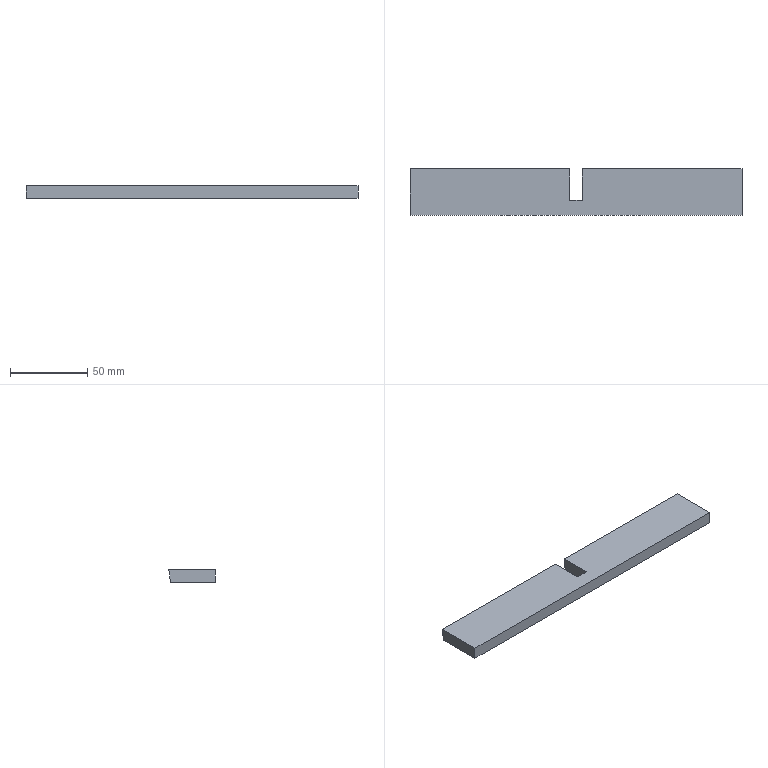Part | SolidWorks | features BaseBody 1 | 1 solid | 10 faces | box 215.2 x 30 x 8 mm | volume 49393 mm3 | plane 10
STEP:
#1=CARTESIAN_POINT('',(4.,15.,8.));
#2=VERTEX_POINT('',#1);
#3=CARTESIAN_POINT('',(4.,13.904,0.));
#4=VERTEX_POINT('',#3);
#5=CARTESIAN_POINT('',(4.,14.452,4.));
#6=DIRECTION('',(0.,-0.1357,-0.9907));
#7=VECTOR('',#6,1000.);
#8=LINE('',#5,#7);
#9=EDGE_CURVE('',#2,#4,#8,.T.);
#10=ORIENTED_EDGE('',*,*,#9,.F.);
#11=CARTESIAN_POINT('',(107.6,15.,8.));
#12=VERTEX_POINT('',#11);
#13=CARTESIAN_POINT('',(55.8,15.,8.));
#14=DIRECTION('',(-1.,0.,0.));
#15=VECTOR('',#14,1000.);
#16=LINE('',#13,#15);
#17=EDGE_CURVE('',#12,#2,#16,.T.);
#18=ORIENTED_EDGE('',*,*,#17,.F.);
#19=CARTESIAN_POINT('',(107.6,13.904,0.));
#20=VERTEX_POINT('',#19);
#21=CARTESIAN_POINT('',(107.6,14.452,4.));
#22=DIRECTION('',(0.,0.1357,0.9907));
#23=VECTOR('',#22,1000.);
#24=LINE('',#21,#23);
#25=EDGE_CURVE('',#20,#12,#24,.T.);
#26=ORIENTED_EDGE('',*,*,#25,.F.);
#27=CARTESIAN_POINT('',(55.8,13.904,0.));
#28=DIRECTION('',(1.,0.,0.));
#29=VECTOR('',#28,1000.);
#30=LINE('',#27,#29);
#31=EDGE_CURVE('',#4,#20,#30,.T.);
#32=ORIENTED_EDGE('',*,*,#31,.F.);
#33=EDGE_LOOP('',(#10,#18,#26,#32));
#34=FACE_OUTER_BOUND('',#33,.T.);
#35=CARTESIAN_POINT('',(4.,15.,8.));
#36=DIRECTION('',(0.,-0.9907,0.1357));
#37=DIRECTION('',(0.,-0.1357,-0.9907));
#38=AXIS2_PLACEMENT_3D('',#35,#36,#37);
#39=PLANE('',#38);
#40=ADVANCED_FACE('',(#34),#39,.F.);
#41=CARTESIAN_POINT('',(-4.,13.904,0.));
#42=VERTEX_POINT('',#41);
#43=CARTESIAN_POINT('',(-4.,-6.596,0.));
#44=VERTEX_POINT('',#43);
#45=CARTESIAN_POINT('',(-4.,-0.5479,0.));
#46=DIRECTION('',(0.,-1.,0.));
#47=VECTOR('',#46,1000.);
#48=LINE('',#45,#47);
#49=EDGE_CURVE('',#42,#44,#48,.T.);
#50=ORIENTED_EDGE('',*,*,#49,.T.);
#51=CARTESIAN_POINT('',(4.,-6.596,0.));
#52=VERTEX_POINT('',#51);
#53=CARTESIAN_POINT('',(0.,-6.596,0.));
#54=DIRECTION('',(1.,0.,0.));
#55=VECTOR('',#54,1000.);
#56=LINE('',#53,#55);
#57=EDGE_CURVE('',#44,#52,#56,.T.);
#58=ORIENTED_EDGE('',*,*,#57,.T.);
#59=CARTESIAN_POINT('',(4.,-0.5479,0.));
#60=DIRECTION('',(0.,1.,0.));
#61=VECTOR('',#60,1000.);
#62=LINE('',#59,#61);
#63=EDGE_CURVE('',#52,#4,#62,.T.);
#64=ORIENTED_EDGE('',*,*,#63,.T.);
#65=ORIENTED_EDGE('',*,*,#31,.T.);
#66=CARTESIAN_POINT('',(107.6,-15.,0.));
#67=VERTEX_POINT('',#66);
#68=CARTESIAN_POINT('',(107.6,-0.5479,0.));
#69=DIRECTION('',(0.,-1.,0.));
#70=VECTOR('',#69,1000.);
#71=LINE('',#68,#70);
#72=EDGE_CURVE('',#20,#67,#71,.T.);
#73=ORIENTED_EDGE('',*,*,#72,.T.);
#74=CARTESIAN_POINT('',(-107.6,-15.,0.));
#75=VERTEX_POINT('',#74);
#76=CARTESIAN_POINT('',(0.,-15.,0.));
#77=DIRECTION('',(-1.,0.,0.));
#78=VECTOR('',#77,1000.);
#79=LINE('',#76,#78);
#80=EDGE_CURVE('',#67,#75,#79,.T.);
#81=ORIENTED_EDGE('',*,*,#80,.T.);
#82=CARTESIAN_POINT('',(-107.6,13.904,0.));
#83=VERTEX_POINT('',#82);
#84=CARTESIAN_POINT('',(-107.6,-0.5479,0.));
#85=DIRECTION('',(0.,1.,0.));
#86=VECTOR('',#85,1000.);
#87=LINE('',#84,#86);
#88=EDGE_CURVE('',#75,#83,#87,.T.);
#89=ORIENTED_EDGE('',*,*,#88,.T.);
#90=CARTESIAN_POINT('',(0.,13.904,0.));
#91=DIRECTION('',(1.,0.,0.));
#92=VECTOR('',#91,1000.);
#93=LINE('',#90,#92);
#94=EDGE_CURVE('',#83,#42,#93,.T.);
#95=ORIENTED_EDGE('',*,*,#94,.T.);
#96=EDGE_LOOP('',(#50,#58,#64,#65,#73,#81,#89,#95));
#97=FACE_OUTER_BOUND('',#96,.T.);
#98=CARTESIAN_POINT('',(107.6,-15.,0.));
#99=DIRECTION('',(0.,0.,-1.));
#100=DIRECTION('',(-1.,0.,0.));
#101=AXIS2_PLACEMENT_3D('',#98,#99,#100);
#102=PLANE('',#101);
#103=ADVANCED_FACE('',(#97),#102,.T.);
#104=CARTESIAN_POINT('',(4.,-5.5,8.));
#105=VERTEX_POINT('',#104);
#106=CARTESIAN_POINT('',(4.,-5.5,8.));
#107=DIRECTION('',(0.,-0.1357,-0.9907));
#108=VECTOR('',#107,1000.);
#109=LINE('',#106,#108);
#110=EDGE_CURVE('',#105,#52,#109,.T.);
#111=ORIENTED_EDGE('',*,*,#110,.F.);
#112=CARTESIAN_POINT('',(4.,4.202,8.));
#113=DIRECTION('',(0.,-1.,0.));
#114=VECTOR('',#113,1000.);
#115=LINE('',#112,#114);
#116=EDGE_CURVE('',#2,#105,#115,.T.);
#117=ORIENTED_EDGE('',*,*,#116,.F.);
#118=ORIENTED_EDGE('',*,*,#9,.T.);
#119=ORIENTED_EDGE('',*,*,#63,.F.);
#120=EDGE_LOOP('',(#111,#117,#118,#119));
#121=FACE_OUTER_BOUND('',#120,.T.);
#122=CARTESIAN_POINT('',(4.,-6.725,8.));
#123=DIRECTION('',(1.,0.,0.));
#124=DIRECTION('',(0.,0.,-1.));
#125=AXIS2_PLACEMENT_3D('',#122,#123,#124);
#126=PLANE('',#125);
#127=ADVANCED_FACE('',(#121),#126,.F.);
#128=ORIENTED_EDGE('',*,*,#116,.T.);
#129=CARTESIAN_POINT('',(-4.,-5.5,8.));
#130=VERTEX_POINT('',#129);
#131=CARTESIAN_POINT('',(0.,-5.5,8.));
#132=DIRECTION('',(1.,0.,0.));
#133=VECTOR('',#132,1000.);
#134=LINE('',#131,#133);
#135=EDGE_CURVE('',#130,#105,#134,.T.);
#136=ORIENTED_EDGE('',*,*,#135,.F.);
#137=CARTESIAN_POINT('',(-4.,15.,8.));
#138=VERTEX_POINT('',#137);
#139=CARTESIAN_POINT('',(-4.,0.,8.));
#140=DIRECTION('',(0.,-1.,0.));
#141=VECTOR('',#140,1000.);
#142=LINE('',#139,#141);
#143=EDGE_CURVE('',#138,#130,#142,.T.);
#144=ORIENTED_EDGE('',*,*,#143,.F.);
#145=CARTESIAN_POINT('',(-107.6,15.,8.));
#146=VERTEX_POINT('',#145);
#147=CARTESIAN_POINT('',(0.,15.,8.));
#148=DIRECTION('',(1.,0.,0.));
#149=VECTOR('',#148,1000.);
#150=LINE('',#147,#149);
#151=EDGE_CURVE('',#146,#138,#150,.T.);
#152=ORIENTED_EDGE('',*,*,#151,.F.);
#153=CARTESIAN_POINT('',(-107.6,-15.,8.));
#154=VERTEX_POINT('',#153);
#155=CARTESIAN_POINT('',(-107.6,0.,8.));
#156=DIRECTION('',(0.,1.,0.));
#157=VECTOR('',#156,1000.);
#158=LINE('',#155,#157);
#159=EDGE_CURVE('',#154,#146,#158,.T.);
#160=ORIENTED_EDGE('',*,*,#159,.F.);
#161=CARTESIAN_POINT('',(107.6,-15.,8.));
#162=VERTEX_POINT('',#161);
#163=CARTESIAN_POINT('',(0.,-15.,8.));
#164=DIRECTION('',(-1.,0.,0.));
#165=VECTOR('',#164,1000.);
#166=LINE('',#163,#165);
#167=EDGE_CURVE('',#162,#154,#166,.T.);
#168=ORIENTED_EDGE('',*,*,#167,.F.);
#169=CARTESIAN_POINT('',(107.6,0.,8.));
#170=DIRECTION('',(0.,-1.,0.));
#171=VECTOR('',#170,1000.);
#172=LINE('',#169,#171);
#173=EDGE_CURVE('',#12,#162,#172,.T.);
#174=ORIENTED_EDGE('',*,*,#173,.F.);
#175=ORIENTED_EDGE('',*,*,#17,.T.);
#176=EDGE_LOOP('',(#128,#136,#144,#152,#160,#168,#174,#175));
#177=FACE_OUTER_BOUND('',#176,.T.);
#178=CARTESIAN_POINT('',(107.6,-15.,8.));
#179=DIRECTION('',(0.,0.,-1.));
#180=DIRECTION('',(-1.,0.,0.));
#181=AXIS2_PLACEMENT_3D('',#178,#179,#180);
#182=PLANE('',#181);
#183=ADVANCED_FACE('',(#177),#182,.F.);
#184=ORIENTED_EDGE('',*,*,#25,.T.);
#185=ORIENTED_EDGE('',*,*,#173,.T.);
#186=CARTESIAN_POINT('',(107.6,-15.,4.));
#187=DIRECTION('',(0.,0.,1.));
#188=VECTOR('',#187,1000.);
#189=LINE('',#186,#188);
#190=EDGE_CURVE('',#67,#162,#189,.T.);
#191=ORIENTED_EDGE('',*,*,#190,.F.);
#192=ORIENTED_EDGE('',*,*,#72,.F.);
#193=EDGE_LOOP('',(#184,#185,#191,#192));
#194=FACE_OUTER_BOUND('',#193,.T.);
#195=CARTESIAN_POINT('',(107.6,-15.,0.));
#196=DIRECTION('',(-1.,0.,0.));
#197=DIRECTION('',(0.,0.,1.));
#198=AXIS2_PLACEMENT_3D('',#195,#196,#197);
#199=PLANE('',#198);
#200=ADVANCED_FACE('',(#194),#199,.F.);
#201=CARTESIAN_POINT('',(-4.,-6.048,4.));
#202=DIRECTION('',(0.,-0.1357,-0.9907));
#203=VECTOR('',#202,1000.);
#204=LINE('',#201,#203);
#205=EDGE_CURVE('',#130,#44,#204,.T.);
#206=ORIENTED_EDGE('',*,*,#205,.F.);
#207=ORIENTED_EDGE('',*,*,#135,.T.);
#208=ORIENTED_EDGE('',*,*,#110,.T.);
#209=ORIENTED_EDGE('',*,*,#57,.F.);
#210=EDGE_LOOP('',(#206,#207,#208,#209));
#211=FACE_OUTER_BOUND('',#210,.T.);
#212=CARTESIAN_POINT('',(-4.,-5.5,8.));
#213=DIRECTION('',(0.,-0.9907,0.1357));
#214=DIRECTION('',(0.,-0.1357,-0.9907));
#215=AXIS2_PLACEMENT_3D('',#212,#213,#214);
#216=PLANE('',#215);
#217=ADVANCED_FACE('',(#211),#216,.F.);
#218=CARTESIAN_POINT('',(-4.,15.,8.));
#219=DIRECTION('',(0.,-0.1357,-0.9907));
#220=VECTOR('',#219,1000.);
#221=LINE('',#218,#220);
#222=EDGE_CURVE('',#138,#42,#221,.T.);
#223=ORIENTED_EDGE('',*,*,#222,.F.);
#224=ORIENTED_EDGE('',*,*,#143,.T.);
#225=ORIENTED_EDGE('',*,*,#205,.T.);
#226=ORIENTED_EDGE('',*,*,#49,.F.);
#227=EDGE_LOOP('',(#223,#224,#225,#226));
#228=FACE_OUTER_BOUND('',#227,.T.);
#229=CARTESIAN_POINT('',(-4.,-6.725,0.));
#230=DIRECTION('',(-1.,0.,0.));
#231=DIRECTION('',(0.,0.,1.));
#232=AXIS2_PLACEMENT_3D('',#229,#230,#231);
#233=PLANE('',#232);
#234=ADVANCED_FACE('',(#228),#233,.F.);
#235=ORIENTED_EDGE('',*,*,#222,.T.);
#236=ORIENTED_EDGE('',*,*,#94,.F.);
#237=CARTESIAN_POINT('',(-107.6,14.452,4.));
#238=DIRECTION('',(0.,-0.1357,-0.9907));
#239=VECTOR('',#238,1000.);
#240=LINE('',#237,#239);
#241=EDGE_CURVE('',#146,#83,#240,.T.);
#242=ORIENTED_EDGE('',*,*,#241,.F.);
#243=ORIENTED_EDGE('',*,*,#151,.T.);
#244=EDGE_LOOP('',(#235,#236,#242,#243));
#245=FACE_OUTER_BOUND('',#244,.T.);
#246=CARTESIAN_POINT('',(-107.6,15.,8.));
#247=DIRECTION('',(0.,-0.9907,0.1357));
#248=DIRECTION('',(0.,-0.1357,-0.9907));
#249=AXIS2_PLACEMENT_3D('',#246,#247,#248);
#250=PLANE('',#249);
#251=ADVANCED_FACE('',(#245),#250,.F.);
#252=ORIENTED_EDGE('',*,*,#241,.T.);
#253=ORIENTED_EDGE('',*,*,#88,.F.);
#254=CARTESIAN_POINT('',(-107.6,-15.,4.));
#255=DIRECTION('',(0.,0.,-1.));
#256=VECTOR('',#255,1000.);
#257=LINE('',#254,#256);
#258=EDGE_CURVE('',#154,#75,#257,.T.);
#259=ORIENTED_EDGE('',*,*,#258,.F.);
#260=ORIENTED_EDGE('',*,*,#159,.T.);
#261=EDGE_LOOP('',(#252,#253,#259,#260));
#262=FACE_OUTER_BOUND('',#261,.T.);
#263=CARTESIAN_POINT('',(-107.6,-15.,8.));
#264=DIRECTION('',(1.,0.,0.));
#265=DIRECTION('',(0.,0.,-1.));
#266=AXIS2_PLACEMENT_3D('',#263,#264,#265);
#267=PLANE('',#266);
#268=ADVANCED_FACE('',(#262),#267,.F.);
#269=ORIENTED_EDGE('',*,*,#190,.T.);
#270=ORIENTED_EDGE('',*,*,#167,.T.);
#271=ORIENTED_EDGE('',*,*,#258,.T.);
#272=ORIENTED_EDGE('',*,*,#80,.F.);
#273=EDGE_LOOP('',(#269,#270,#271,#272));
#274=FACE_OUTER_BOUND('',#273,.T.);
#275=CARTESIAN_POINT('',(107.6,-15.,0.));
#276=DIRECTION('',(0.,1.,0.));
#277=DIRECTION('',(-1.,0.,0.));
#278=AXIS2_PLACEMENT_3D('',#275,#276,#277);
#279=PLANE('',#278);
#280=ADVANCED_FACE('',(#274),#279,.F.);
#281=CLOSED_SHELL('',(#40,#103,#127,#183,#200,#217,#234,#251,#268,#280));
#282=MANIFOLD_SOLID_BREP('',#281);
#283=CARTESIAN_POINT('',(0.,0.,0.));
#284=DIRECTION('',(0.,0.,1.));
#285=DIRECTION('',(1.,0.,0.));
#286=AXIS2_PLACEMENT_3D('',#283,#284,#285);
#287=(LENGTH_UNIT()NAMED_UNIT(*)SI_UNIT(.MILLI.,.METRE.));
#288=UNCERTAINTY_MEASURE_WITH_UNIT(LENGTH_MEASURE(0.00001),#287,'','');
#289=(NAMED_UNIT(*)PLANE_ANGLE_UNIT()SI_UNIT($,.RADIAN.));
#290=(NAMED_UNIT(*)SI_UNIT($,.STERADIAN.)SOLID_ANGLE_UNIT());
#291=(GEOMETRIC_REPRESENTATION_CONTEXT(3)GLOBAL_UNCERTAINTY_ASSIGNED_CONTEXT((#288))GLOBAL_UNIT_ASSIGNED_CONTEXT((#287,#289,#290))REPRESENTATION_CONTEXT('',''));
#292=ADVANCED_BREP_SHAPE_REPRESENTATION('',(#282,#286),#291);